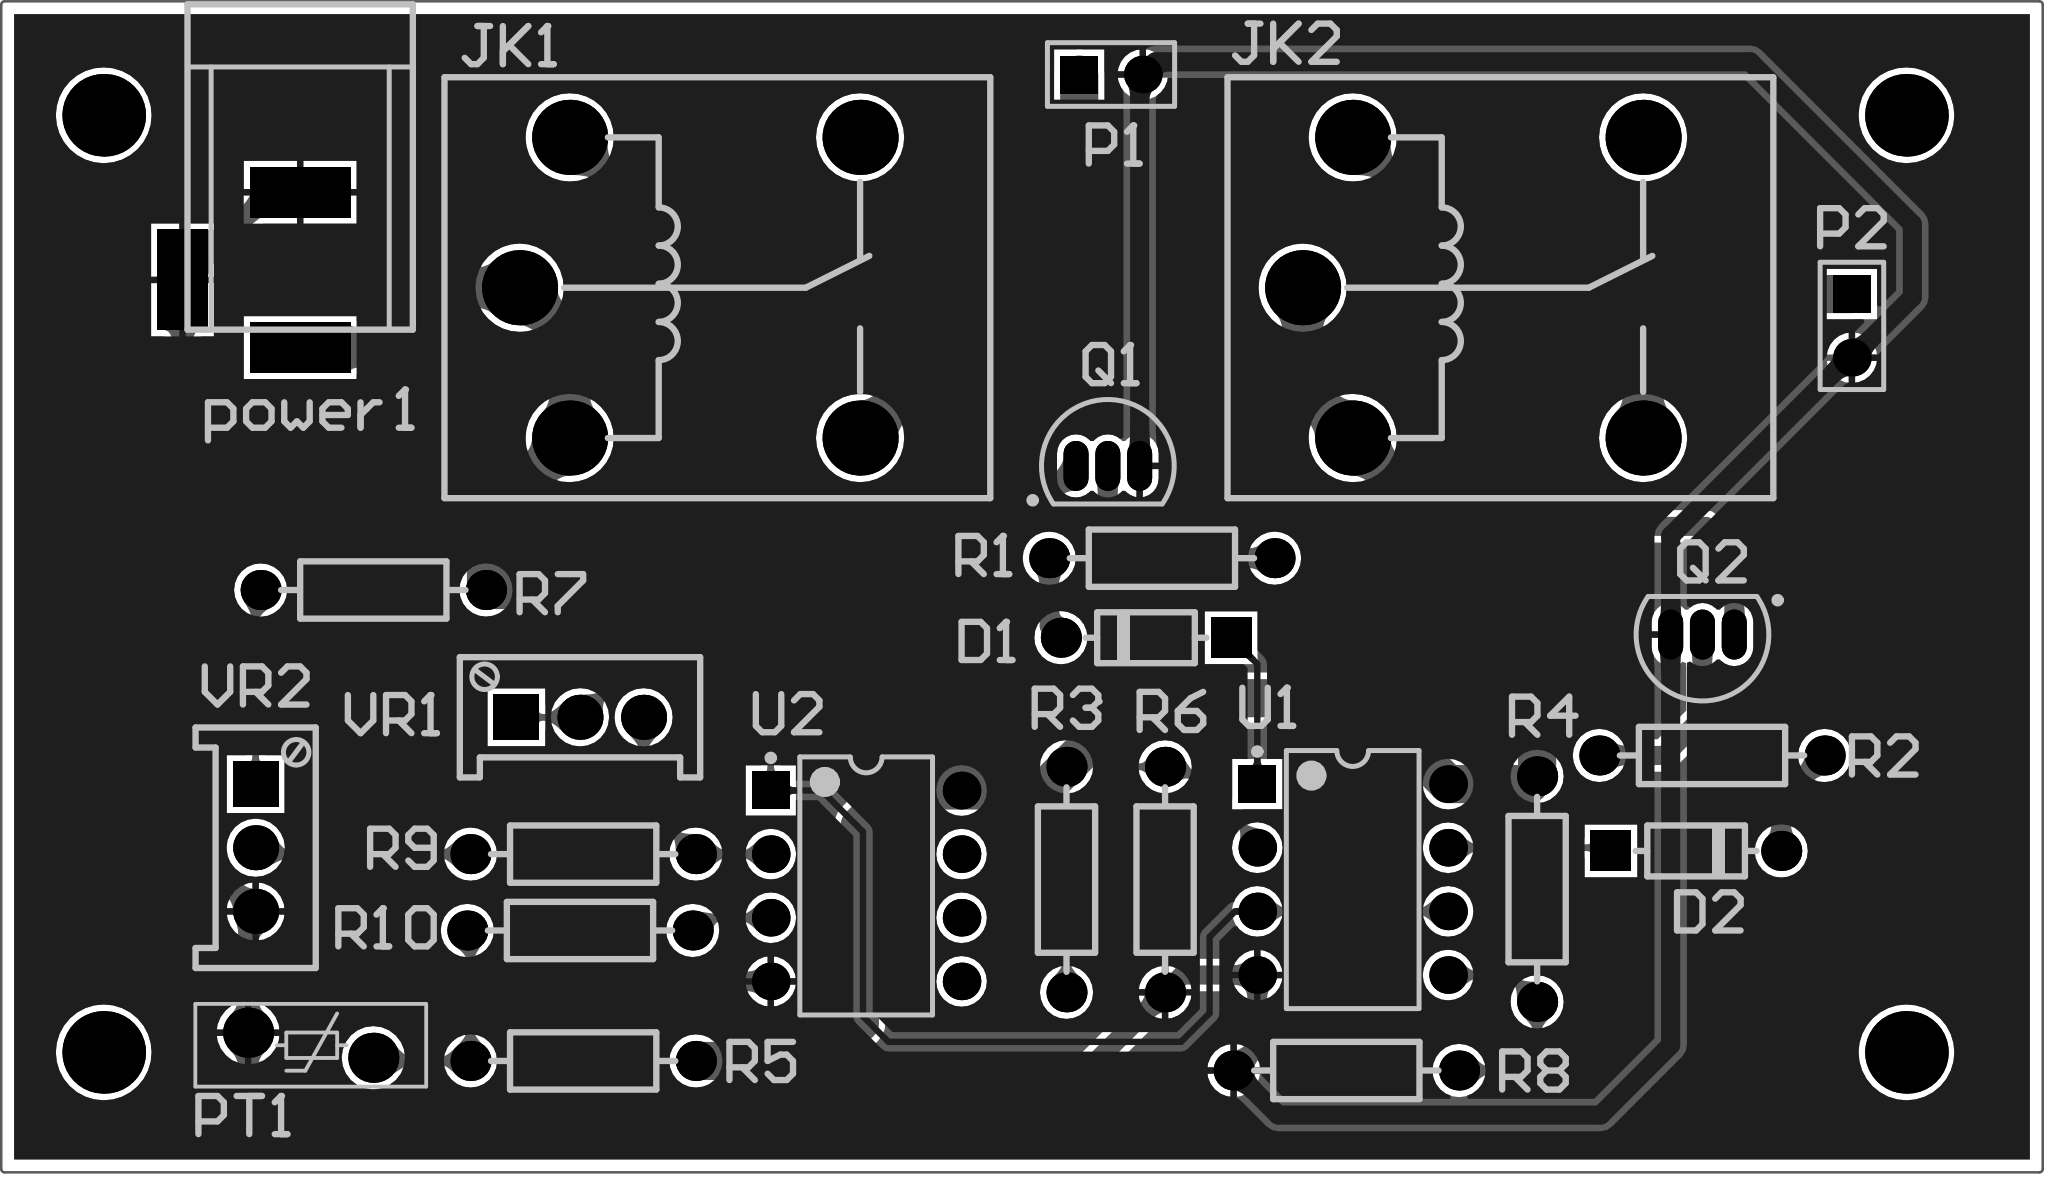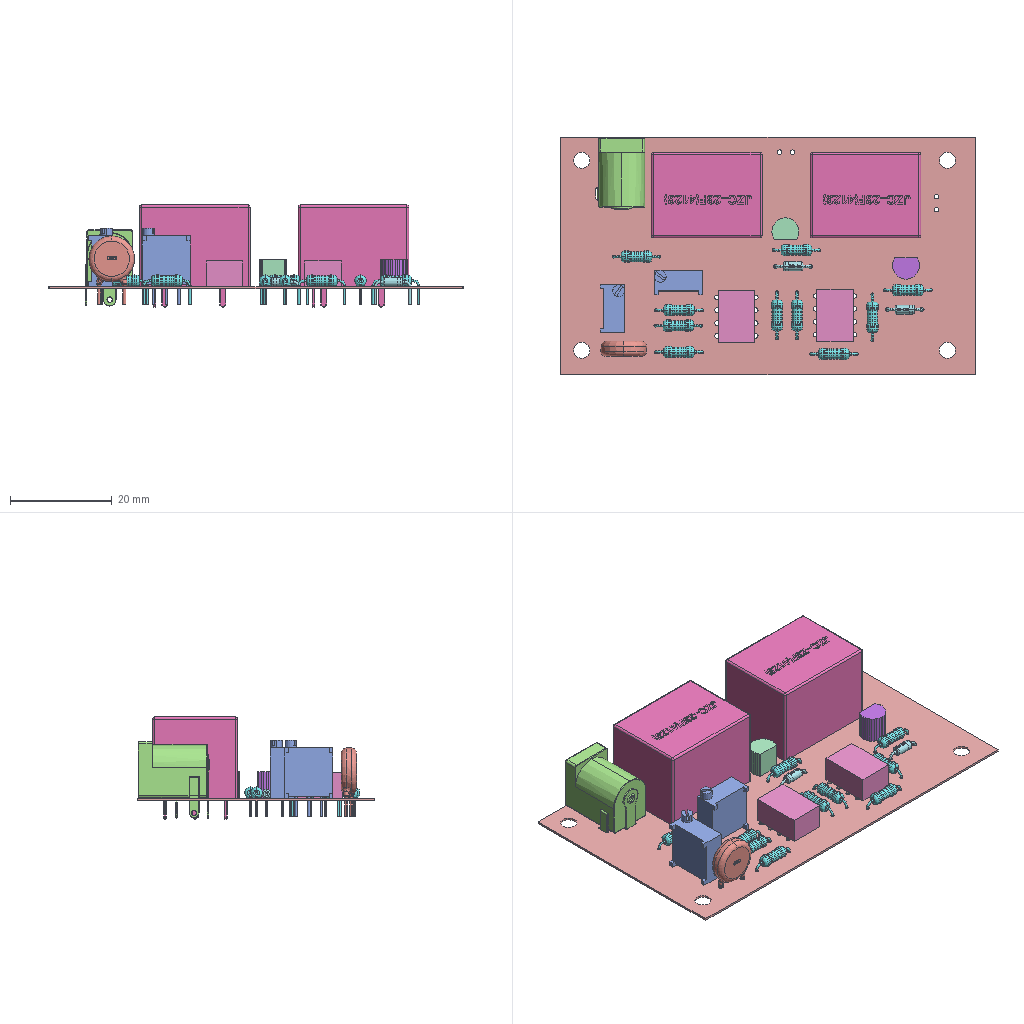Circuit board layout | Altium Designer | box 81.5 x 46.7 x 20.1 mm
Layer stack:
# Altium Designer layer stack of  (unit mm; dielectric type: 0 none, 1 core, 2 prepreg, 3 surface material)
index,name,kind,layer,copper_thickness_mm,dielectric_type,dielectric_thickness_mm,dielectric_material,dielectric_constant
0,Top Paste,other,,,,,,
1,Top Overlay,other,,,,,,
2,Top Solder,dielectric,,,3,0.0102,Solder Resist,3.5
3,Top Layer,copper,Top Layer,0.0356,,,,
4,Dielectric 1,dielectric,,,0,0.32,FR-4,4.8
5,Bottom Layer,copper,Bottom Layer,0.0356,,,,
6,Bottom Solder,dielectric,,,3,0.0102,Solder Resist,3.5
7,Bottom Overlay,other,,,,,,
8,Bottom Paste,other,,,,,,
# drill layer pairs: low layer,high layer
drill_pair,Top Layer,Bottom Layer
Part placement:
Designator,Comment,Layer,Footprint,Center-X(mm),Center-Y(mm),Rotation
VR2,200R,TopLayer,3296W,36.068,66.167,270
VR1,100k,TopLayer,3296W,49.022,71.374,360
U2,AD823AN,TopLayer,DIP-8,60.452,64.643,0
U1,AD823AN,TopLayer,DIP-8,79.883,64.897,0
R10,1k,TopLayer,RS_1/4W,49.022,62.865,180
R9,1k,TopLayer,RS_1/4W,49.149,65.913,180
R8,250R,TopLayer,RS_1/4W,79.629,57.277,360
R7,2k,TopLayer,RS_1/4W,40.767,76.454,360
R6,1.64k,TopLayer,RS_1/4W,72.39,64.897,90
R5,2k,TopLayer,RS_1/4W,49.149,57.658,360
R4,11.75k,TopLayer,RS_1/4W,87.249,64.516,90
R3,10.36k,TopLayer,RS_1/4W,68.453,64.897,90
R2,5k,TopLayer,RS_1/4W,94.234,69.85,360
R1,5k,TopLayer,RS_1/4W,72.263,77.724,180
Q2,NPN,TopLayer,TO-226-AA,93.853,74.676,90
Q1,NPN,TopLayer,TO-226-AA,70.104,81.407,270
PT1,PT100,TopLayer,VDR_9D-4.5,38.267,58.285,360
power1,,TopLayer,DC-005,35.496,89.229,90
P2,加热棒,TopLayer,HDR1X2,99.822,86.995,270
P1,风扇,TopLayer,HDR1X2,70.231,97.028,360
JK2,JZC-23F(12VDC),TopLayer,JZC-23F(4123),84.683,88.519,360
JK1,JZC-23F(12VDC),TopLayer,JZC-23F(4123),53.409,88.519,360
D2,1N4148,TopLayer,DO-35,93.599,66.04,360
D1,1N4148,TopLayer,DO-35,71.628,74.549,180
Pad and via stacks:
# Altium Designer via and pad stacks of  (unit mm). Each distinct definition once, with the count of objects using it.
# via: kind,start_layer,end_layer,hole_mm,diameter_mm,mode(0 simple;1 top-mid-bottom;2 full stack),diameter_per_layer,count,example_net
# pad: kind,layer,hole_mm,hole_type(0 round;1 square;2 slot),plating,top_size,top_shape(1 round;2 rect;3 octagon;9 rounded rect),mid_size,bottom_size,mode,footprint,size_per_layer,count,example
pad,Multi-Layer,3.2,0,plated,3.3x3.3,1,3.3x3.3,3.3x3.3,0,,,4,3
pad,Multi-Layer,0.9,0,plated,2x1,1,2x1,2x1,0,TO-226-AA,,6,Q2.1
pad,Multi-Layer,1.6,0,plated,3x3,1,3x3,3x3,0,JZC-23F(4123),,10,JK1.2
pad,Multi-Layer,0.9,0,plated,1.5x1.5,2,1.5x1.5,1.5x1.5,0,HDR1X2,,2,P1.1
pad,Multi-Layer,0.9,0,plated,1.5x1.5,1,1.5x1.5,1.5x1.5,0,HDR1X2,,2,P1.2
pad,Multi-Layer,0.8,0,plated,1.6x1.6,1,1.6x1.6,1.6x1.6,0,DO-35,,2,D1.2
pad,Multi-Layer,0.8,0,plated,1.6x1.6,2,1.6x1.6,1.6x1.6,0,DO-35,,2,D1.1
pad,Multi-Layer,0.6,0,plated,1.6x1.6,1,1.6x1.6,1.6x1.6,0,RS 1/4W,,20,R1.2
pad,Multi-Layer,0.8,2,plated,2x4,2,2x4,2x4,0,DC-005,,2,power1.1
pad,Multi-Layer,0.8,2,plated,4x2,2,4x2,4x2,0,DC-005,,1,power1.3
pad,Multi-Layer,0.9,0,plated,1.5x1.5,2,1.5x1.5,1.5x1.5,0,DIP-8,,2,U1.1
pad,Multi-Layer,0.9,0,plated,1.5x1.5,1,1.5x1.5,1.5x1.5,0,DIP-8,,14,U1.2
pad,Multi-Layer,0.7,0,plated,1.8x1.8,1,1.8x1.8,1.8x1.8,0,3296W,,4,VR1.3
pad,Multi-Layer,0.7,0,plated,1.8x1.8,2,1.8x1.8,1.8x1.8,0,3296W,,2,VR1.1
pad,Multi-Layer,1,0,plated,2x2,1,2x2,2x2,0,VDR 9D-4.5,,2,PT1.2
Copper pours:
name,layer,net,type(0 solid;1 hatched;2 none)
D,Top Layer,GND,0
D,Bottom Layer,GND,0
Design rules, without the lines most boards share:
# Altium Designer design rules of  (exported by Altium Designer, unit mm)
# columns: name | kind | enabled | priority | scope1 | scope2 | descriptor | typed fields (field=value)
SilkToSilkClearance | 55 | enabled | 1 | All | All | Silk to Silk (Clearance=0mil) (All),(All) |
SilkToSolderMaskClearance | 54 | enabled | 1 | IsPad | All | Silk To Solder Mask (Clearance=0mil) (IsPad),(All) |
MinimumSolderMaskSliver | 53 | enabled | 1 | All | All | Minimum Solder Mask Sliver (Gap=0mil) (All),(All) |
HoleToHoleClearance | 52 | enabled | 1 | All | All | Hole To Hole Clearance (Gap=10mil) (All),(All) | gap=0.254
DiffPairsRouting | 51 | enabled | 1 | All | All | Differential Pairs Uncoupled Length using the Gap Constraints (Min=10mil) (Max=10mil) (Prefered=10mil)  and Width Constraints (Min=15mil) (Max=15mil) (Prefered=15mil) (All) |
HoleSize | 42 | enabled | 1 | All | All | Hole Size Constraint (Min=1mil) (Max=1000mil) (All) |
SolderMaskExpansion | 13 | enabled | 1 | All | All | Solder Mask Expansion (Expansion =4mil) (All) | expansion=0.1016
PasteMaskExpansion | 14 | enabled | 1 | All | All | Paste Mask Expansion (Expansion =0mil) (All) | expansion=0
RoutingVias | 11 | enabled | 1 | All | All | Routing Via (MinHoleWidth=28mil) (MaxHoleWidth=28mil) (PreferredHoleWidth=28mil) (MinWidth=50mil) (MaxWidth=50mil) (PreferedWidth=50mil) (All) | via_min_hole=0.7112 via_max_hole=0.7112 via_preferred_diameter=1.27 via_preferred_hole=0.7112
Width | 2 | enabled | 1 | All | All | Width Constraint (Min=10mil) (Max=60mil) (Preferred=10mil) (All) |
PolygonConnect | 20 | enabled | 1 | All | All | Polygon Connect Rule(Relief Connect )(Conductor Width=10mil) (Relief Angle=90 Angle) (Entries=4) (Air Gap Width=10mil) (All),(All) | connect_style(0=relief,1=direct,2=none)=0 relief_conductor_width=0.254 relief_entries=4
PlaneConnect | 6 | enabled | 1 | All | All | Power Plane Connect Rule(Relief Connect )(Expansion=20mil) (Conductor Width=10mil) (Air Gap=10mil) (Entries=4) (All) | relief_conductor_width=0.254 relief_entries=4 relief_expansion=0.508
Clearance | 0 | enabled | 1 | All | All | Clearance Constraint (Gap=10mil) (All),(All) | gap=0.254